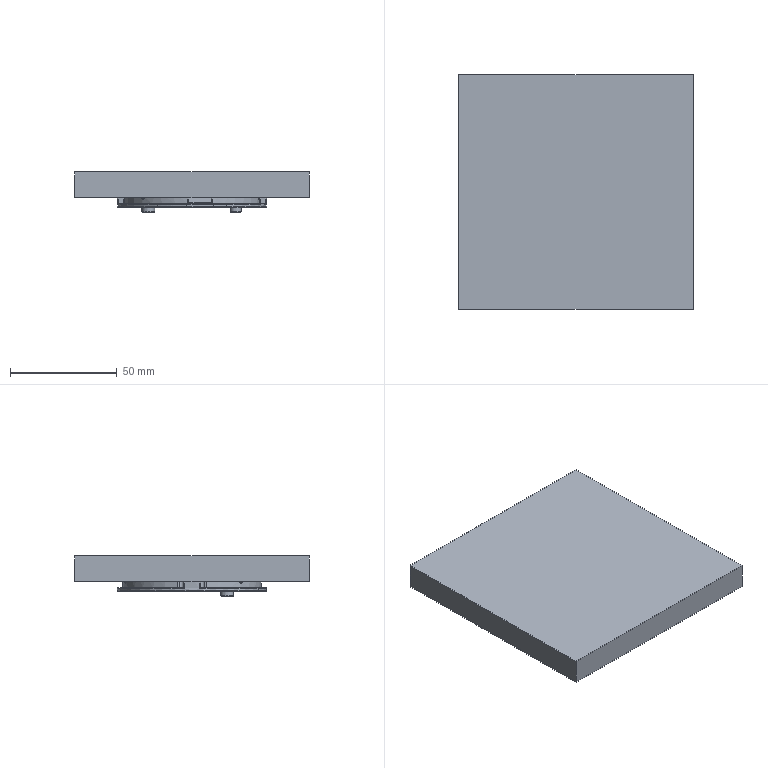NC program | NX | posted with a generic post | part box 110 x 110 x 18.8 mm
Lines 7770 to 8004 of 8004:
(ZLEVEL_PROFILE_COPY_COPY_COPY_1_COPY , TOOL : D4A45)
N15484 T21 M6
N15486 G54
N15488 G17 G0 G90 X-20.75 Y-16.5 S9500 M3
N15490 G43 Z30. H21
N15492 Z1.
N15494 G94 G1 Z-1. F1000.
N15496 G3 X-20.5 Y-16.75 R0.25
N15498 X-20.75 Y-16.5 R-0.25
N15500 X-20.65 Y-16.673 R0.2
N15502 G1 Z0.
N15504 G0 Z30.
N15506 X20.75 Y-16.5
N15508 Z1.
N15510 G1 Z-1.
N15512 G3 X20.5 Y-16.25 R0.25
N15514 X20.75 Y-16.5 R-0.25
N15516 X20.65 Y-16.327 R0.2
N15518 G1 Z0.
N15520 G0 Z30.
N15522 X25.052 Y-15.835
N15524 Z0.
N15526 G1 Z-1.
N15528 X24.5 Y-16.154
N15530 G3 X24.3 Y-16.5 R0.4
N15532 G2 X20.5 Y-20.3 R3.8
N15534 X24.3 Y-16.5 R-3.8
N15536 G3 X24.5 Y-16.846 R0.4
N15538 G1 X25.052 Y-17.165
N15540 Z0.
N15542 G0 Z30.
N15544 X-24.546 Y-17.162
N15546 Z0.
N15548 G1 Z-1.
N15550 X-24. Y-16.846
N15552 G3 X-23.8 Y-16.5 R0.4
N15554 G2 X-20.5 Y-13.2 R3.3
N15556 X-23.8 Y-16.5 R-3.3
N15558 G3 X-24. Y-16.154 R0.4
N15560 G1 X-24.546 Y-15.838
N15562 Z0.
N15564 G0 Z30.
(ZLEVEL_PROFILE_COPY_COPY_COPY_1_COPY_COPY , TOOL : D4A45)
N15566 X-16.95 Y17.
N15568 Z-1.3
N15570 G1 Z-3.3
N15572 Y-8.144
N15574 G3 X-16.579 Y-8.247 R0.2
N15576 G2 X-16.093 Y-7.544 R6.8
N15578 G1 X-16.06 Y-7.51
N15580 X-16.045 Y-7.466
N15582 X-16.05 Y-7.42
N15584 Y17.
N15586 G3 X-16.25 Y17.2 R0.2
N15588 G1 X-16.75
N15590 G3 X-16.95 Y17. R0.2
N15592 G1 X-16.953 Y16.946
N15594 X-16.923 Y16.9
N15596 Z-2.3
N15598 G0 Z30.
N15600 X-20.8 Y-11.508
N15602 Z-1.3
N15604 G1 Z-3.3
N15606 Y17.
N15608 G3 X-21. Y17.2 R0.2
N15610 G1 X-21.5
N15612 G3 X-21.7 Y17. R0.2
N15614 G1 Y-11.644
N15616 G3 X-21.5 Y-11.99 R0.4
N15618 G1 Z-2.3
N15620 G0 Z30.
N15622 X-12.2 Y17.
N15624 Z-1.3
N15626 G1 Z-3.3
N15628 Y-4.863
N15630 G3 X-11.964 Y-5.059 R0.2
N15632 G2 X-11.479 Y-4.989 R6.8
N15634 G3 X-11.3 Y-4.79 R0.2
N15636 G1 Y17.
N15638 G3 X-11.5 Y17.2 R0.2
N15640 G1 X-12.
N15642 G3 X-12.2 Y17. R0.2
N15644 G1 X-12.203 Y16.946
N15646 X-12.173 Y16.9
N15648 Z-2.3
N15650 G0 Z30.
N15652 X11.49 Y-8.431
N15654 Z-2.3
N15656 G1 Z-3.3
N15658 X11.096 Y-7.75
N15660 G3 X10.75 Y-7.55 R0.4
N15662 G1 X-10.75
N15664 G3 X-14.95 Y-11.75 R4.2
N15666 G1 Y-21.25
N15668 G3 X-10.75 Y-25.45 R4.2
N15670 G1 X-10.
N15672 G2 X-8.2 Y-27.25 R1.8
N15674 G1 Y-32.496
N15676 G2 X-10.529 Y-34.217 R1.8
N15678 X2.632 Y-35.703 R-35.8
N15680 X0.7 Y-33.908 R1.8
N15682 G1 Y-27.25
N15684 G2 X2.5 Y-25.45 R1.8
N15686 G1 X10.75
N15688 G3 X14.95 Y-21.25 R4.2
N15690 G1 Y-11.75
N15692 G3 X10.75 Y-7.55 R4.2
N15694 X10.404 Y-7.75 R0.4
N15696 G1 X10.057 Y-8.35
N15698 Z-2.3
N15700 G0 Z30.
(ZLEVEL_PROFILE_COPY_COPY_COPY_1_COPY_COPY_COPY , TOOL : D4A45)
N15702 X-12.95 Y-15.9
N15704 Z-4.3
N15706 G1 Z-5.3
N15708 X-13.589 Y-16.5
N15710 G3 X-13.242 Y-16.7 R0.4
N15712 G1 X-12.
N15714 G3 X-11.8 Y-16.5 R0.2
N15716 G1 Y-9.499
N15718 G3 X-12. Y-9.152 R0.4
N15720 G1 X-12.6 Y-10.559
N15722 Z-4.3
N15724 G0 Z30.
N15726 X-7.9 Y-9.55
N15728 Z-4.3
N15730 G1 Z-5.3
N15732 X-8.5 Y-8.905
N15734 G3 X-8.7 Y-9.252 R0.4
N15736 G1 Y-18.
N15738 G2 X-10.5 Y-19.8 R1.8
N15740 G1 X-13.245
N15742 G3 X-13.591 Y-20. R0.4
N15744 G1 X-12.95 Y-20.6
N15746 Z-4.3
N15748 G0 Z30.
N15750 M5
(ZLEVEL_PROFILE_1_COPY_1_COPY_1 , TOOL : R0.75)
N15752 T13 M6
N15754 G54
N15756 G17 G0 G90 X0.902 Y4.98 S37561 M3
N15758 G43 Z30. H13
N15760 Z-1.8
N15762 G94 G1 X2.196 Z-1.868 F800.
N15764 Y5.086 Z-1.873
N15766 X-0.134 Z-1.995
N15768 X-0.206 Z-1.999
N15770 X-0.322 Y5.155 Z-2.006
N15772 X-0.39 Y5.272 Z-2.013
N15774 X-0.389 Y5.344 Z-2.017
N15776 Y9.937 Z-2.258
N15778 X-0.623 Z-2.27
N15780 Y7.458 Z-2.4
N15782 Y4.98 F1000.
N15784 X2.196
N15786 Y5.086
N15788 X-0.134
N15790 G2 X-0.389 Y5.344 R0.257
N15792 G1 Y9.937
N15794 X-0.623
N15796 Y7.458
N15798 Y4.98 Z-2.443
N15800 X2.133 Z-2.491
N15802 X2.196 Z-2.492
N15804 Y4.998 Z-2.493
N15806 Y5.016
N15808 Y5.086 Z-2.494
N15810 X1.87 Z-2.5
N15812 X-0.134
N15814 G2 X-0.389 Y5.344 R0.257
N15816 G1 Y9.937
N15818 X-0.623
N15820 Y7.458
N15822 Y4.98 Z-2.543
N15824 X2.133 Z-2.591
N15826 X2.196 Z-2.592
N15828 Y4.998 Z-2.593
N15830 Y5.016
N15832 Y5.086 Z-2.594
N15834 X1.87 Z-2.6
N15836 X-0.139
N15838 G2 X-0.389 Y5.336 R0.25
N15840 G1 Y9.937
N15842 X-0.623
N15844 Y4.98
N15846 X2.196
N15848 Y5.086
N15850 X1.87
N15852 Z-2.1
N15854 G0 Z30.
N15856 M5
(CUTTERCOMP , TOOL : D3)
N15858 T17 M6
N15860 G54
N15862 G17 G0 G90 X26.562 Y-15.474 S9500 M3
N15864 G43 Z30. H17
N15866 Z-0.8
N15868 G94 G1 Z-2.3 F1000.
N15870 G41 X26.468 Y-15.508 D17
N15872 X25.2 Y-16.24
N15874 G3 X25.05 Y-16.5 R0.3
N15876 G2 X20.5 Y-21.05 R4.55
N15878 X25.05 Y-16.5 R-4.55
N15880 G3 X25.2 Y-16.76 R0.3
N15882 G1 X26.468 Y-17.492
N15884 G40
N15886 X26.562 Y-17.526
N15888 Z-0.8
N15890 G0 Z30.
N15892 X-26.055 Y-17.522
N15894 Z-0.8
N15896 G1 Z-2.3
N15898 G41 X-25.961 Y-17.488
N15900 X-24.7 Y-16.76
N15902 G3 X-24.55 Y-16.5 R0.3
N15904 G2 X-20.5 Y-12.45 R4.05
N15906 X-24.55 Y-16.5 R-4.05
N15908 G3 X-24.7 Y-16.24 R0.3
N15910 G1 X-25.961 Y-15.512
N15912 G40
N15914 X-26.055 Y-15.478
N15916 Z-0.8
N15918 G0 Z30.
N15920 M5
N15922 M2